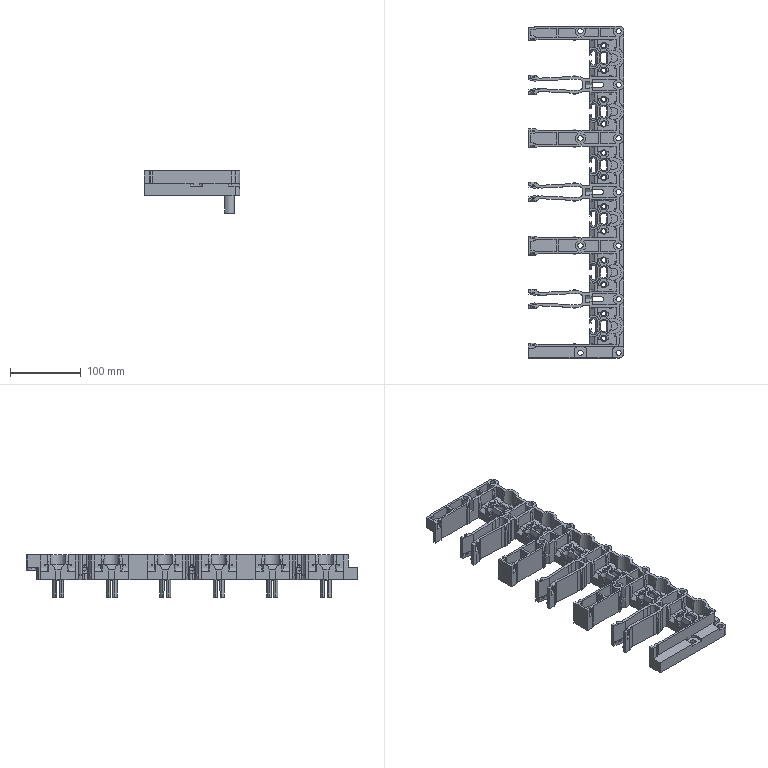Part | SolidWorks | features BaseBody 1 | 1 solid | 1811 faces | box 135.78 x 470.75 x 59.95 mm | volume 480051 mm3 | plane 1159 | cylinder 628 | cone 24 | commonest cylinder face diameters 14.8 x69 12.277 x48 2 x42 14.7 x30 6.3 x24 8 x24